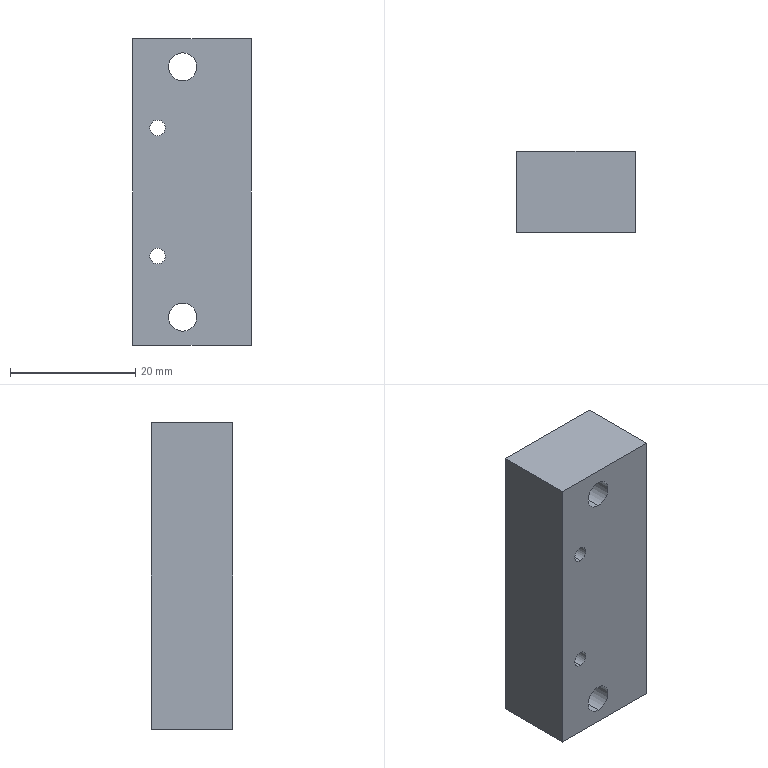Part | STEP file | PN_0003 sensor seat | 1 solid | 20 faces | box 19 x 13 x 49 mm | volume 11246 mm3 | cylinder 12 | plane 8 | commonest cylinder face diameters 2.5 x4 4.5 x4 8 x4